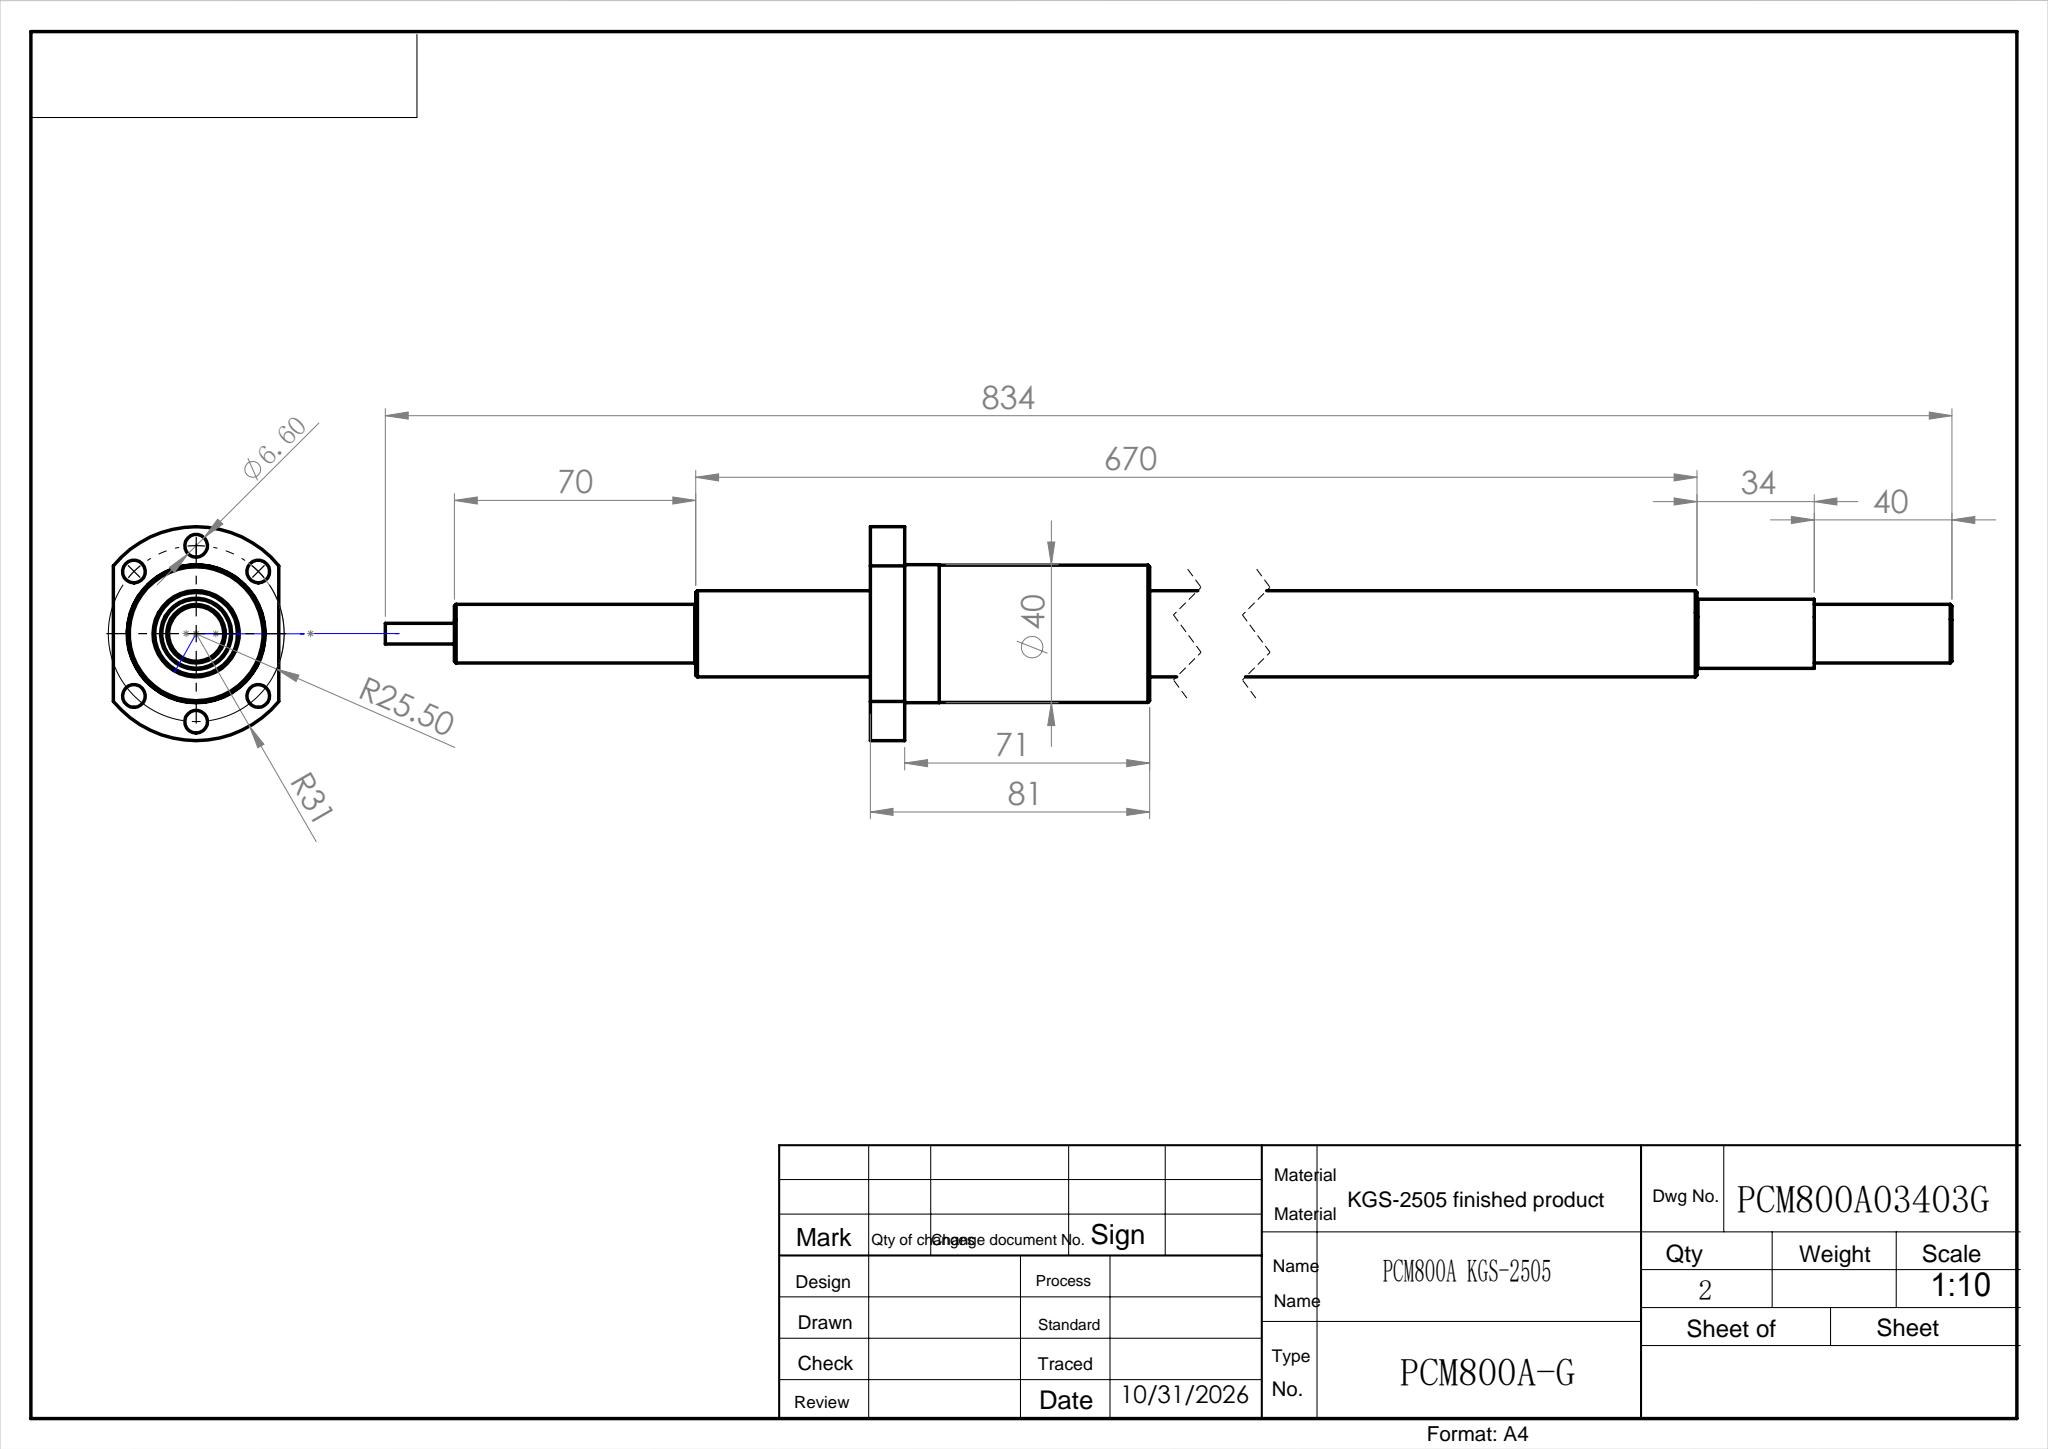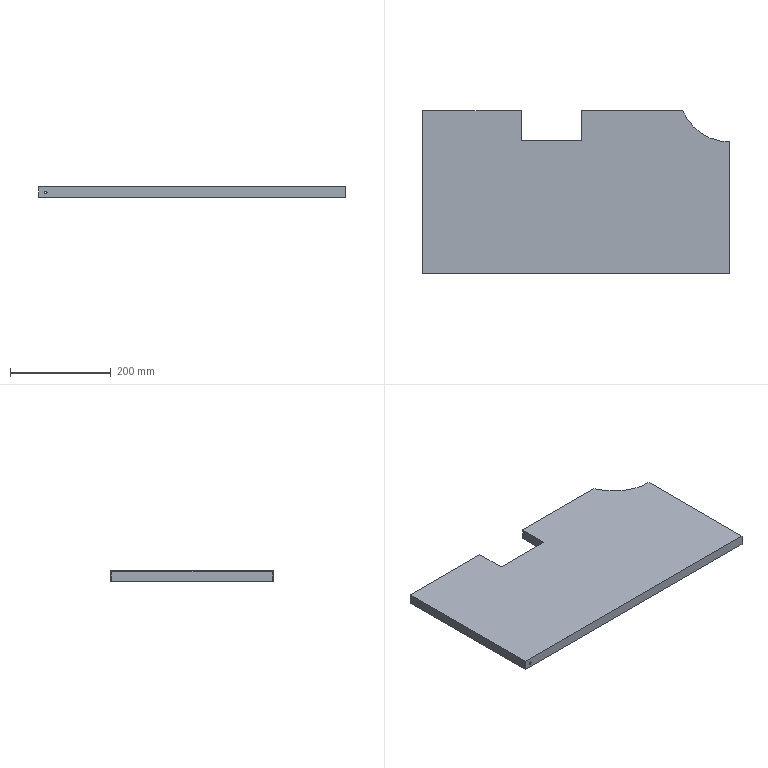Part | SolidWorks | features ICE 3, Extrusion 1, Shell 1 | 1 solid | 41 faces | box 609 x 323 x 20 mm | volume 440064 mm3 | cylinder 22 | plane 19 | commonest cylinder face diameters 5.5 x20 200 x1 204 x1